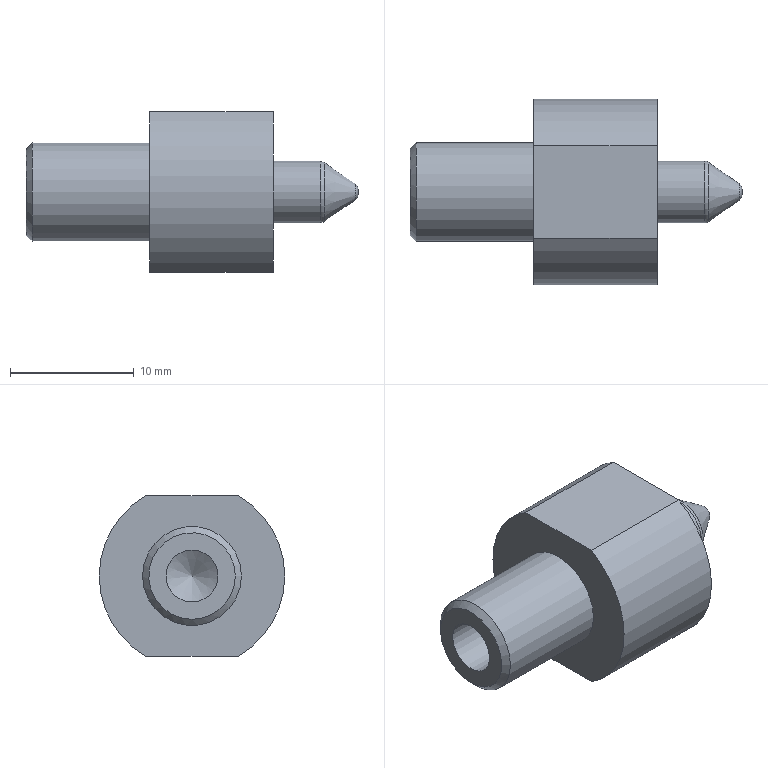Part | NX | features BREP 1 | 1 solid | 16 faces | box 26.856 x 15 x 13 mm | volume 2090 mm3 | plane 6 | cylinder 5 | cone 3 | torus 2 | commonest cylinder face diameters 15 x2 4.2 x1 5 x1 8 x1
STEP:
#1=CARTESIAN_POINT('',(6.572,3.742,6.5));
#2=VERTEX_POINT('',#1);
#3=CARTESIAN_POINT('',(6.572,3.742,-6.5));
#4=VERTEX_POINT('',#3);
#5=CARTESIAN_POINT('',(6.572,0.,0.));
#6=DIRECTION('',(-1.,0.,0.));
#7=DIRECTION('',(0.,-1.,0.));
#8=AXIS2_PLACEMENT_3D('',#5,#6,#7);
#9=CIRCLE('',#8,7.5);
#10=EDGE_CURVE('',#2,#4,#9,.T.);
#11=ORIENTED_EDGE('',*,*,#10,.T.);
#12=CARTESIAN_POINT('',(-3.428,3.742,-6.5));
#13=VERTEX_POINT('',#12);
#14=CARTESIAN_POINT('',(-13.428,3.742,-6.5));
#15=DIRECTION('',(-1.,0.,0.));
#16=VECTOR('',#15,1000.);
#17=LINE('',#14,#16);
#18=EDGE_CURVE('',#4,#13,#17,.T.);
#19=ORIENTED_EDGE('',*,*,#18,.T.);
#20=CARTESIAN_POINT('',(-3.428,3.742,6.5));
#21=VERTEX_POINT('',#20);
#22=CARTESIAN_POINT('',(-3.428,0.,0.));
#23=DIRECTION('',(1.,0.,0.));
#24=DIRECTION('',(0.,-1.,0.));
#25=AXIS2_PLACEMENT_3D('',#22,#23,#24);
#26=CIRCLE('',#25,7.5);
#27=EDGE_CURVE('',#13,#21,#26,.T.);
#28=ORIENTED_EDGE('',*,*,#27,.T.);
#29=CARTESIAN_POINT('',(-13.428,3.742,6.5));
#30=DIRECTION('',(1.,0.,0.));
#31=VECTOR('',#30,1000.);
#32=LINE('',#29,#31);
#33=EDGE_CURVE('',#21,#2,#32,.T.);
#34=ORIENTED_EDGE('',*,*,#33,.T.);
#35=EDGE_LOOP('',(#11,#19,#28,#34));
#36=FACE_BOUND('',#35,.T.);
#37=CARTESIAN_POINT('',(-13.428,0.,0.));
#38=DIRECTION('',(-1.,0.,0.));
#39=DIRECTION('',(0.,1.,0.));
#40=AXIS2_PLACEMENT_3D('',#37,#38,#39);
#41=CYLINDRICAL_SURFACE('',#40,7.5);
#42=ADVANCED_FACE('',(#36),#41,.T.);
#43=CARTESIAN_POINT('',(-3.428,-3.742,-6.5));
#44=VERTEX_POINT('',#43);
#45=CARTESIAN_POINT('',(6.572,-3.742,-6.5));
#46=VERTEX_POINT('',#45);
#47=CARTESIAN_POINT('',(13.428,-3.742,-6.5));
#48=DIRECTION('',(1.,0.,0.));
#49=VECTOR('',#48,1000.);
#50=LINE('',#47,#49);
#51=EDGE_CURVE('',#44,#46,#50,.T.);
#52=ORIENTED_EDGE('',*,*,#51,.F.);
#53=CARTESIAN_POINT('',(-3.428,6.891,-6.5));
#54=DIRECTION('',(0.,-1.,0.));
#55=VECTOR('',#54,1000.);
#56=LINE('',#53,#55);
#57=EDGE_CURVE('',#13,#44,#56,.T.);
#58=ORIENTED_EDGE('',*,*,#57,.F.);
#59=ORIENTED_EDGE('',*,*,#18,.F.);
#60=CARTESIAN_POINT('',(6.572,6.891,-6.5));
#61=DIRECTION('',(0.,1.,0.));
#62=VECTOR('',#61,1000.);
#63=LINE('',#60,#62);
#64=EDGE_CURVE('',#46,#4,#63,.T.);
#65=ORIENTED_EDGE('',*,*,#64,.F.);
#66=EDGE_LOOP('',(#52,#58,#59,#65));
#67=FACE_BOUND('',#66,.T.);
#68=CARTESIAN_POINT('',(13.428,6.891,-6.5));
#69=DIRECTION('',(0.,0.,1.));
#70=DIRECTION('',(0.,1.,0.));
#71=AXIS2_PLACEMENT_3D('',#68,#69,#70);
#72=PLANE('',#71);
#73=ADVANCED_FACE('',(#67),#72,.F.);
#74=CARTESIAN_POINT('',(6.572,-2.5,0.));
#75=VERTEX_POINT('',#74);
#76=CARTESIAN_POINT('',(6.572,0.,0.));
#77=DIRECTION('',(1.,0.,0.));
#78=DIRECTION('',(0.,-1.,0.));
#79=AXIS2_PLACEMENT_3D('',#76,#77,#78);
#80=CIRCLE('',#79,2.5);
#81=EDGE_CURVE('',#75,#75,#80,.T.);
#82=ORIENTED_EDGE('',*,*,#81,.F.);
#83=EDGE_LOOP('',(#82));
#84=FACE_BOUND('',#83,.T.);
#85=CARTESIAN_POINT('',(6.572,-3.742,6.5));
#86=VERTEX_POINT('',#85);
#87=CARTESIAN_POINT('',(6.572,2.5,6.5));
#88=DIRECTION('',(0.,1.,0.));
#89=VECTOR('',#88,1000.);
#90=LINE('',#87,#89);
#91=EDGE_CURVE('',#86,#2,#90,.T.);
#92=ORIENTED_EDGE('',*,*,#91,.F.);
#93=CARTESIAN_POINT('',(6.572,0.,0.));
#94=DIRECTION('',(-1.,0.,0.));
#95=DIRECTION('',(0.,-1.,0.));
#96=AXIS2_PLACEMENT_3D('',#93,#94,#95);
#97=CIRCLE('',#96,7.5);
#98=EDGE_CURVE('',#46,#86,#97,.T.);
#99=ORIENTED_EDGE('',*,*,#98,.F.);
#100=ORIENTED_EDGE('',*,*,#64,.T.);
#101=ORIENTED_EDGE('',*,*,#10,.F.);
#102=EDGE_LOOP('',(#92,#99,#100,#101));
#103=FACE_BOUND('',#102,.T.);
#104=CARTESIAN_POINT('',(6.572,2.5,0.));
#105=DIRECTION('',(-1.,0.,0.));
#106=DIRECTION('',(0.,1.,0.));
#107=AXIS2_PLACEMENT_3D('',#104,#105,#106);
#108=PLANE('',#107);
#109=ADVANCED_FACE('',(#84,#103),#108,.F.);
#110=ORIENTED_EDGE('',*,*,#33,.F.);
#111=CARTESIAN_POINT('',(-3.428,-3.742,6.5));
#112=VERTEX_POINT('',#111);
#113=CARTESIAN_POINT('',(-3.428,-7.709,6.5));
#114=DIRECTION('',(0.,1.,0.));
#115=VECTOR('',#114,1000.);
#116=LINE('',#113,#115);
#117=EDGE_CURVE('',#112,#21,#116,.T.);
#118=ORIENTED_EDGE('',*,*,#117,.F.);
#119=CARTESIAN_POINT('',(13.428,-3.742,6.5));
#120=DIRECTION('',(-1.,0.,0.));
#121=VECTOR('',#120,1000.);
#122=LINE('',#119,#121);
#123=EDGE_CURVE('',#86,#112,#122,.T.);
#124=ORIENTED_EDGE('',*,*,#123,.F.);
#125=ORIENTED_EDGE('',*,*,#91,.T.);
#126=EDGE_LOOP('',(#110,#118,#124,#125));
#127=FACE_BOUND('',#126,.T.);
#128=CARTESIAN_POINT('',(13.428,-7.709,6.5));
#129=DIRECTION('',(0.,0.,-1.));
#130=DIRECTION('',(0.,-1.,0.));
#131=AXIS2_PLACEMENT_3D('',#128,#129,#130);
#132=PLANE('',#131);
#133=ADVANCED_FACE('',(#127),#132,.F.);
#134=CARTESIAN_POINT('',(-3.428,0.,0.));
#135=DIRECTION('',(1.,0.,0.));
#136=DIRECTION('',(0.,-1.,0.));
#137=AXIS2_PLACEMENT_3D('',#134,#135,#136);
#138=CIRCLE('',#137,7.5);
#139=EDGE_CURVE('',#112,#44,#138,.T.);
#140=ORIENTED_EDGE('',*,*,#139,.F.);
#141=ORIENTED_EDGE('',*,*,#117,.T.);
#142=ORIENTED_EDGE('',*,*,#27,.F.);
#143=ORIENTED_EDGE('',*,*,#57,.T.);
#144=EDGE_LOOP('',(#140,#141,#142,#143));
#145=FACE_BOUND('',#144,.T.);
#146=CARTESIAN_POINT('',(-3.428,-4.,0.));
#147=VERTEX_POINT('',#146);
#148=CARTESIAN_POINT('',(-3.428,0.,0.));
#149=DIRECTION('',(-1.,0.,0.));
#150=DIRECTION('',(0.,-1.,0.));
#151=AXIS2_PLACEMENT_3D('',#148,#149,#150);
#152=CIRCLE('',#151,4.);
#153=EDGE_CURVE('',#147,#147,#152,.T.);
#154=ORIENTED_EDGE('',*,*,#153,.F.);
#155=EDGE_LOOP('',(#154));
#156=FACE_BOUND('',#155,.T.);
#157=CARTESIAN_POINT('',(-3.428,7.5,0.));
#158=DIRECTION('',(1.,0.,0.));
#159=DIRECTION('',(0.,-1.,0.));
#160=AXIS2_PLACEMENT_3D('',#157,#158,#159);
#161=PLANE('',#160);
#162=ADVANCED_FACE('',(#145,#156),#161,.F.);
#163=ORIENTED_EDGE('',*,*,#139,.T.);
#164=ORIENTED_EDGE('',*,*,#51,.T.);
#165=ORIENTED_EDGE('',*,*,#98,.T.);
#166=ORIENTED_EDGE('',*,*,#123,.T.);
#167=EDGE_LOOP('',(#163,#164,#165,#166));
#168=FACE_BOUND('',#167,.T.);
#169=CARTESIAN_POINT('',(-13.428,0.,0.));
#170=DIRECTION('',(-1.,0.,0.));
#171=DIRECTION('',(0.,1.,0.));
#172=AXIS2_PLACEMENT_3D('',#169,#170,#171);
#173=CYLINDRICAL_SURFACE('',#172,7.5);
#174=ADVANCED_FACE('',(#168),#173,.T.);
#175=ORIENTED_EDGE('',*,*,#81,.T.);
#176=EDGE_LOOP('',(#175));
#177=FACE_BOUND('',#176,.T.);
#178=CARTESIAN_POINT('',(10.414,-2.5,0.));
#179=VERTEX_POINT('',#178);
#180=CARTESIAN_POINT('',(10.414,0.,0.));
#181=DIRECTION('',(-1.,0.,0.));
#182=DIRECTION('',(0.,-1.,0.));
#183=AXIS2_PLACEMENT_3D('',#180,#181,#182);
#184=CIRCLE('',#183,2.5);
#185=EDGE_CURVE('',#179,#179,#184,.T.);
#186=ORIENTED_EDGE('',*,*,#185,.T.);
#187=EDGE_LOOP('',(#186));
#188=FACE_BOUND('',#187,.T.);
#189=CARTESIAN_POINT('',(-13.428,0.,0.));
#190=DIRECTION('',(-1.,0.,0.));
#191=DIRECTION('',(0.,1.,0.));
#192=AXIS2_PLACEMENT_3D('',#189,#190,#191);
#193=CYLINDRICAL_SURFACE('',#192,2.5);
#194=ADVANCED_FACE('',(#177,#188),#193,.T.);
#195=CARTESIAN_POINT('',(-12.928,-4.,0.));
#196=VERTEX_POINT('',#195);
#197=CARTESIAN_POINT('',(-12.928,0.,0.));
#198=DIRECTION('',(1.,0.,0.));
#199=DIRECTION('',(0.,-1.,0.));
#200=AXIS2_PLACEMENT_3D('',#197,#198,#199);
#201=CIRCLE('',#200,4.);
#202=EDGE_CURVE('',#196,#196,#201,.T.);
#203=ORIENTED_EDGE('',*,*,#202,.T.);
#204=EDGE_LOOP('',(#203));
#205=FACE_BOUND('',#204,.T.);
#206=ORIENTED_EDGE('',*,*,#153,.T.);
#207=EDGE_LOOP('',(#206));
#208=FACE_BOUND('',#207,.T.);
#209=CARTESIAN_POINT('',(-13.428,0.,0.));
#210=DIRECTION('',(-1.,0.,0.));
#211=DIRECTION('',(0.,1.,0.));
#212=AXIS2_PLACEMENT_3D('',#209,#210,#211);
#213=CYLINDRICAL_SURFACE('',#212,4.);
#214=ADVANCED_FACE('',(#205,#208),#213,.T.);
#215=CARTESIAN_POINT('',(10.701,2.41,0.));
#216=VERTEX_POINT('',#215);
#217=CARTESIAN_POINT('',(10.701,0.,0.));
#218=DIRECTION('',(-1.,0.,0.));
#219=DIRECTION('',(0.,1.,0.));
#220=AXIS2_PLACEMENT_3D('',#217,#218,#219);
#221=CIRCLE('',#220,2.41);
#222=EDGE_CURVE('',#216,#216,#221,.T.);
#223=ORIENTED_EDGE('',*,*,#222,.T.);
#224=EDGE_LOOP('',(#223));
#225=FACE_BOUND('',#224,.T.);
#226=ORIENTED_EDGE('',*,*,#185,.F.);
#227=EDGE_LOOP('',(#226));
#228=FACE_BOUND('',#227,.T.);
#229=CARTESIAN_POINT('',(10.414,0.,0.));
#230=DIRECTION('',(1.,0.,0.));
#231=DIRECTION('',(0.,0.,-1.));
#232=AXIS2_PLACEMENT_3D('',#229,#230,#231);
#233=TOROIDAL_SURFACE('',#232,2.,0.5);
#234=ADVANCED_FACE('',(#225,#228),#233,.T.);
#235=ORIENTED_EDGE('',*,*,#202,.F.);
#236=EDGE_LOOP('',(#235));
#237=FACE_BOUND('',#236,.T.);
#238=CARTESIAN_POINT('',(-13.428,0.,-3.5));
#239=VERTEX_POINT('',#238);
#240=CARTESIAN_POINT('',(-13.428,0.,0.));
#241=DIRECTION('',(1.,0.,0.));
#242=DIRECTION('',(0.,0.,-1.));
#243=AXIS2_PLACEMENT_3D('',#240,#241,#242);
#244=CIRCLE('',#243,3.5);
#245=EDGE_CURVE('',#239,#239,#244,.T.);
#246=ORIENTED_EDGE('',*,*,#245,.T.);
#247=EDGE_LOOP('',(#246));
#248=FACE_BOUND('',#247,.T.);
#249=CARTESIAN_POINT('',(-12.928,0.,0.));
#250=DIRECTION('',(1.,0.,0.));
#251=DIRECTION('',(0.,0.,1.));
#252=AXIS2_PLACEMENT_3D('',#249,#250,#251);
#253=CONICAL_SURFACE('',#252,4.,0.7854);
#254=ADVANCED_FACE('',(#237,#248),#253,.T.);
#255=ORIENTED_EDGE('',*,*,#222,.F.);
#256=EDGE_LOOP('',(#255));
#257=FACE_BOUND('',#256,.T.);
#258=CARTESIAN_POINT('',(13.215,-0.6493,0.));
#259=VERTEX_POINT('',#258);
#260=CARTESIAN_POINT('',(13.215,0.,0.));
#261=DIRECTION('',(-1.,0.,0.));
#262=DIRECTION('',(0.,-1.,0.));
#263=AXIS2_PLACEMENT_3D('',#260,#261,#262);
#264=CIRCLE('',#263,0.6493);
#265=EDGE_CURVE('',#259,#259,#264,.T.);
#266=ORIENTED_EDGE('',*,*,#265,.T.);
#267=EDGE_LOOP('',(#266));
#268=FACE_BOUND('',#267,.T.);
#269=CARTESIAN_POINT('',(10.701,0.,0.));
#270=DIRECTION('',(-1.,0.,0.));
#271=DIRECTION('',(0.,0.,-1.));
#272=AXIS2_PLACEMENT_3D('',#269,#270,#271);
#273=CONICAL_SURFACE('',#272,2.41,0.6109);
#274=ADVANCED_FACE('',(#257,#268),#273,.T.);
#275=CARTESIAN_POINT('',(-13.428,0.,2.1));
#276=VERTEX_POINT('',#275);
#277=CARTESIAN_POINT('',(-13.428,0.,0.));
#278=DIRECTION('',(-1.,0.,0.));
#279=DIRECTION('',(0.,0.,1.));
#280=AXIS2_PLACEMENT_3D('',#277,#278,#279);
#281=CIRCLE('',#280,2.1);
#282=EDGE_CURVE('',#276,#276,#281,.T.);
#283=ORIENTED_EDGE('',*,*,#282,.F.);
#284=EDGE_LOOP('',(#283));
#285=FACE_BOUND('',#284,.T.);
#286=ORIENTED_EDGE('',*,*,#245,.F.);
#287=EDGE_LOOP('',(#286));
#288=FACE_BOUND('',#287,.T.);
#289=CARTESIAN_POINT('',(-13.428,4.,0.));
#290=DIRECTION('',(1.,0.,0.));
#291=DIRECTION('',(0.,-1.,0.));
#292=AXIS2_PLACEMENT_3D('',#289,#290,#291);
#293=PLANE('',#292);
#294=ADVANCED_FACE('',(#285,#288),#293,.F.);
#295=ORIENTED_EDGE('',*,*,#265,.F.);
#296=EDGE_LOOP('',(#295));
#297=FACE_BOUND('',#296,.T.);
#298=CARTESIAN_POINT('',(13.428,-0.2397,0.));
#299=VERTEX_POINT('',#298);
#300=CARTESIAN_POINT('',(13.428,0.2397,0.));
#301=VERTEX_POINT('',#300);
#302=CARTESIAN_POINT('',(13.428,0.,0.));
#303=DIRECTION('',(-1.,0.,0.));
#304=DIRECTION('',(0.,0.,1.));
#305=AXIS2_PLACEMENT_3D('',#302,#303,#304);
#306=CIRCLE('',#305,0.2397);
#307=EDGE_CURVE('',#299,#301,#306,.T.);
#308=ORIENTED_EDGE('',*,*,#307,.T.);
#309=CARTESIAN_POINT('',(13.428,0.,0.));
#310=DIRECTION('',(-1.,0.,0.));
#311=DIRECTION('',(0.,0.,1.));
#312=AXIS2_PLACEMENT_3D('',#309,#310,#311);
#313=CIRCLE('',#312,0.2397);
#314=EDGE_CURVE('',#301,#299,#313,.T.);
#315=ORIENTED_EDGE('',*,*,#314,.T.);
#316=EDGE_LOOP('',(#308,#315));
#317=FACE_BOUND('',#316,.T.);
#318=CARTESIAN_POINT('',(12.928,0.,0.));
#319=DIRECTION('',(-1.,0.,0.));
#320=DIRECTION('',(0.,0.,1.));
#321=AXIS2_PLACEMENT_3D('',#318,#319,#320);
#322=DEGENERATE_TOROIDAL_SURFACE('',#321,0.2397,0.5,.T.);
#323=ADVANCED_FACE('',(#297,#317),#322,.T.);
#324=CARTESIAN_POINT('',(-1.028,0.,2.1));
#325=VERTEX_POINT('',#324);
#326=CARTESIAN_POINT('',(-1.028,0.,0.));
#327=DIRECTION('',(-1.,0.,0.));
#328=DIRECTION('',(0.,0.,1.));
#329=AXIS2_PLACEMENT_3D('',#326,#327,#328);
#330=CIRCLE('',#329,2.1);
#331=EDGE_CURVE('',#325,#325,#330,.T.);
#332=ORIENTED_EDGE('',*,*,#331,.F.);
#333=EDGE_LOOP('',(#332));
#334=FACE_BOUND('',#333,.T.);
#335=ORIENTED_EDGE('',*,*,#282,.T.);
#336=EDGE_LOOP('',(#335));
#337=FACE_BOUND('',#336,.T.);
#338=CARTESIAN_POINT('',(-13.428,0.,0.));
#339=DIRECTION('',(-1.,0.,0.));
#340=DIRECTION('',(0.,0.,-1.));
#341=AXIS2_PLACEMENT_3D('',#338,#339,#340);
#342=CYLINDRICAL_SURFACE('',#341,2.1);
#343=ADVANCED_FACE('',(#334,#337),#342,.F.);
#344=ORIENTED_EDGE('',*,*,#307,.F.);
#345=ORIENTED_EDGE('',*,*,#314,.F.);
#346=EDGE_LOOP('',(#344,#345));
#347=FACE_BOUND('',#346,.T.);
#348=CARTESIAN_POINT('',(13.428,0.,0.));
#349=DIRECTION('',(-1.,0.,0.));
#350=DIRECTION('',(0.,1.,0.));
#351=AXIS2_PLACEMENT_3D('',#348,#349,#350);
#352=PLANE('',#351);
#353=ADVANCED_FACE('',(#347),#352,.F.);
#354=CARTESIAN_POINT('',(0.2337,0.,0.));
#355=VERTEX_POINT('',#354);
#356=VERTEX_LOOP('',#355);
#357=FACE_BOUND('',#356,.T.);
#358=ORIENTED_EDGE('',*,*,#331,.T.);
#359=EDGE_LOOP('',(#358));
#360=FACE_BOUND('',#359,.T.);
#361=CARTESIAN_POINT('',(-1.028,0.,0.));
#362=DIRECTION('',(-1.,0.,0.));
#363=DIRECTION('',(0.,0.,-1.));
#364=AXIS2_PLACEMENT_3D('',#361,#362,#363);
#365=CONICAL_SURFACE('',#364,2.1,1.03);
#366=ADVANCED_FACE('',(#357,#360),#365,.F.);
#367=CLOSED_SHELL('',(#42,#73,#109,#133,#162,#174,#194,#214,#234,#254,#274,#294,#323,#343,#353,#366));
#368=MANIFOLD_SOLID_BREP('',#367);
#369=(LENGTH_UNIT()NAMED_UNIT(*)SI_UNIT(.MILLI.,.METRE.));
#370=UNCERTAINTY_MEASURE_WITH_UNIT(LENGTH_MEASURE(0.00001),#369,'','');
#371=(NAMED_UNIT(*)PLANE_ANGLE_UNIT()SI_UNIT($,.RADIAN.));
#372=(NAMED_UNIT(*)SI_UNIT($,.STERADIAN.)SOLID_ANGLE_UNIT());
#373=(GEOMETRIC_REPRESENTATION_CONTEXT(3)GLOBAL_UNCERTAINTY_ASSIGNED_CONTEXT((#370))GLOBAL_UNIT_ASSIGNED_CONTEXT((#369,#371,#372))REPRESENTATION_CONTEXT('',''));
#374=ADVANCED_BREP_SHAPE_REPRESENTATION('',(#368),#373);